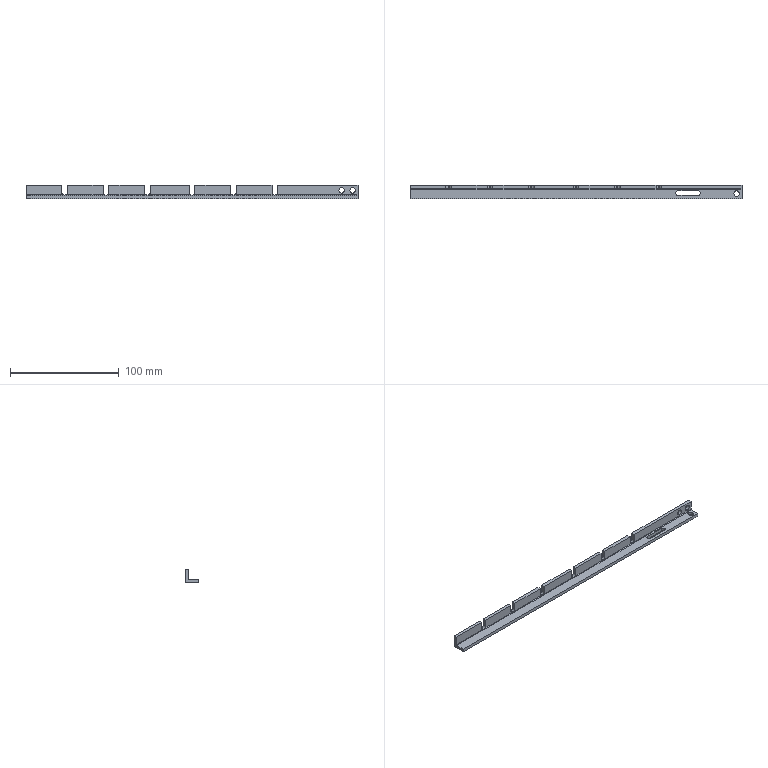Part | SolidWorks | features BaseBody 1 | 1 solid | 85 faces | box 305 x 12 x 12 mm | volume 18035 mm3 | plane 40 | cylinder 33 | spline 12 | commonest cylinder face diameters 4 x14 1 x13 5 x6